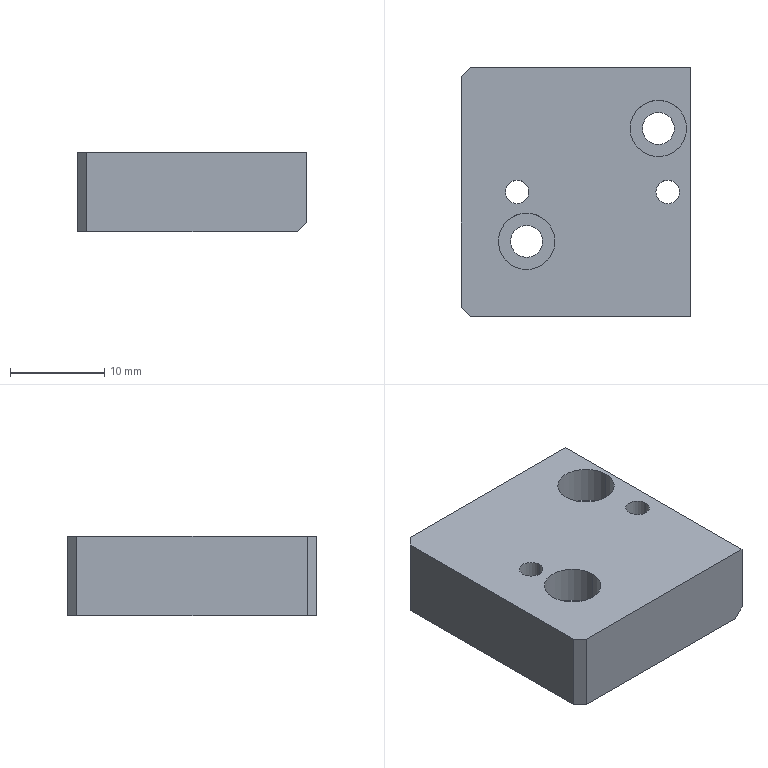Part | SolidWorks | features MoveFace 4, Chamfer 2, DelFace 2, HoleWzd 2, Extrusion 1, Fillet 1, ICE 1 | 1 solid | 30 faces | box 24.4 x 26.5 x 8.5 mm | volume 3196 mm3 | plane 16 | cylinder 14 | commonest cylinder face diameters 2.5 x4 3.4 x4 6 x4 5 x2
STEP:
#1=CARTESIAN_POINT('',(-21.3,93.75,0.));
#2=VERTEX_POINT('',#1);
#3=CARTESIAN_POINT('',(-18.8,93.75,0.));
#4=VERTEX_POINT('',#3);
#5=CARTESIAN_POINT('',(-20.05,93.75,0.));
#6=DIRECTION('',(0.,0.,1.));
#7=DIRECTION('',(1.,0.,0.));
#8=AXIS2_PLACEMENT_3D('',#5,#6,#7);
#9=CIRCLE('',#8,1.25);
#10=EDGE_CURVE('',#2,#4,#9,.T.);
#11=ORIENTED_EDGE('',*,*,#10,.F.);
#12=CARTESIAN_POINT('',(-21.3,93.75,5.));
#13=VERTEX_POINT('',#12);
#14=CARTESIAN_POINT('',(-21.3,93.75,5.));
#15=DIRECTION('',(0.,0.,1.));
#16=VECTOR('',#15,1000.);
#17=LINE('',#14,#16);
#18=EDGE_CURVE('',#2,#13,#17,.T.);
#19=ORIENTED_EDGE('',*,*,#18,.T.);
#20=CARTESIAN_POINT('',(-18.8,93.75,5.));
#21=VERTEX_POINT('',#20);
#22=CARTESIAN_POINT('',(-20.05,93.75,5.));
#23=DIRECTION('',(0.,0.,1.));
#24=DIRECTION('',(1.,0.,0.));
#25=AXIS2_PLACEMENT_3D('',#22,#23,#24);
#26=CIRCLE('',#25,1.25);
#27=EDGE_CURVE('',#13,#21,#26,.T.);
#28=ORIENTED_EDGE('',*,*,#27,.T.);
#29=CARTESIAN_POINT('',(-18.8,93.75,5.));
#30=DIRECTION('',(0.,0.,1.));
#31=VECTOR('',#30,1000.);
#32=LINE('',#29,#31);
#33=EDGE_CURVE('',#4,#21,#32,.T.);
#34=ORIENTED_EDGE('',*,*,#33,.F.);
#35=EDGE_LOOP('',(#11,#19,#28,#34));
#36=FACE_OUTER_BOUND('',#35,.T.);
#37=CARTESIAN_POINT('',(-20.05,93.75,5.));
#38=DIRECTION('',(0.,0.,1.));
#39=DIRECTION('',(1.,0.,0.));
#40=AXIS2_PLACEMENT_3D('',#37,#38,#39);
#41=CYLINDRICAL_SURFACE('',#40,1.25);
#42=ADVANCED_FACE('',(#36),#41,.F.);
#43=CARTESIAN_POINT('',(-5.3,93.75,0.));
#44=VERTEX_POINT('',#43);
#45=CARTESIAN_POINT('',(-2.8,93.75,0.));
#46=VERTEX_POINT('',#45);
#47=CARTESIAN_POINT('',(-4.05,93.75,0.));
#48=DIRECTION('',(0.,0.,1.));
#49=DIRECTION('',(1.,0.,0.));
#50=AXIS2_PLACEMENT_3D('',#47,#48,#49);
#51=CIRCLE('',#50,1.25);
#52=EDGE_CURVE('',#44,#46,#51,.T.);
#53=ORIENTED_EDGE('',*,*,#52,.F.);
#54=CARTESIAN_POINT('',(-5.3,93.75,5.));
#55=VERTEX_POINT('',#54);
#56=CARTESIAN_POINT('',(-5.3,93.75,5.));
#57=DIRECTION('',(0.,0.,1.));
#58=VECTOR('',#57,1000.);
#59=LINE('',#56,#58);
#60=EDGE_CURVE('',#44,#55,#59,.T.);
#61=ORIENTED_EDGE('',*,*,#60,.T.);
#62=CARTESIAN_POINT('',(-2.8,93.75,5.));
#63=VERTEX_POINT('',#62);
#64=CARTESIAN_POINT('',(-4.05,93.75,5.));
#65=DIRECTION('',(0.,0.,1.));
#66=DIRECTION('',(1.,0.,0.));
#67=AXIS2_PLACEMENT_3D('',#64,#65,#66);
#68=CIRCLE('',#67,1.25);
#69=EDGE_CURVE('',#55,#63,#68,.T.);
#70=ORIENTED_EDGE('',*,*,#69,.T.);
#71=CARTESIAN_POINT('',(-2.8,93.75,5.));
#72=DIRECTION('',(0.,0.,1.));
#73=VECTOR('',#72,1000.);
#74=LINE('',#71,#73);
#75=EDGE_CURVE('',#46,#63,#74,.T.);
#76=ORIENTED_EDGE('',*,*,#75,.F.);
#77=EDGE_LOOP('',(#53,#61,#70,#76));
#78=FACE_OUTER_BOUND('',#77,.T.);
#79=CARTESIAN_POINT('',(-4.05,93.75,5.));
#80=DIRECTION('',(0.,0.,1.));
#81=DIRECTION('',(1.,0.,0.));
#82=AXIS2_PLACEMENT_3D('',#79,#80,#81);
#83=CYLINDRICAL_SURFACE('',#82,1.25);
#84=ADVANCED_FACE('',(#78),#83,.F.);
#85=CARTESIAN_POINT('',(-8.05,100.5,1.));
#86=VERTEX_POINT('',#85);
#87=CARTESIAN_POINT('',(-2.05,100.5,1.));
#88=VERTEX_POINT('',#87);
#89=CARTESIAN_POINT('',(-5.05,100.5,1.));
#90=DIRECTION('',(0.,0.,1.));
#91=DIRECTION('',(1.,0.,0.));
#92=AXIS2_PLACEMENT_3D('',#89,#90,#91);
#93=CIRCLE('',#92,3.);
#94=EDGE_CURVE('',#86,#88,#93,.T.);
#95=ORIENTED_EDGE('',*,*,#94,.F.);
#96=CARTESIAN_POINT('',(-8.05,100.5,5.));
#97=VERTEX_POINT('',#96);
#98=CARTESIAN_POINT('',(-8.05,100.5,5.));
#99=DIRECTION('',(0.,0.,1.));
#100=VECTOR('',#99,1000.);
#101=LINE('',#98,#100);
#102=EDGE_CURVE('',#86,#97,#101,.T.);
#103=ORIENTED_EDGE('',*,*,#102,.T.);
#104=CARTESIAN_POINT('',(-2.05,100.5,5.));
#105=VERTEX_POINT('',#104);
#106=CARTESIAN_POINT('',(-5.05,100.5,5.));
#107=DIRECTION('',(0.,0.,1.));
#108=DIRECTION('',(1.,0.,0.));
#109=AXIS2_PLACEMENT_3D('',#106,#107,#108);
#110=CIRCLE('',#109,3.);
#111=EDGE_CURVE('',#97,#105,#110,.T.);
#112=ORIENTED_EDGE('',*,*,#111,.T.);
#113=CARTESIAN_POINT('',(-2.05,100.5,5.));
#114=DIRECTION('',(0.,0.,1.));
#115=VECTOR('',#114,1000.);
#116=LINE('',#113,#115);
#117=EDGE_CURVE('',#88,#105,#116,.T.);
#118=ORIENTED_EDGE('',*,*,#117,.F.);
#119=EDGE_LOOP('',(#95,#103,#112,#118));
#120=FACE_OUTER_BOUND('',#119,.T.);
#121=CARTESIAN_POINT('',(-5.05,100.5,5.));
#122=DIRECTION('',(0.,0.,1.));
#123=DIRECTION('',(1.,0.,0.));
#124=AXIS2_PLACEMENT_3D('',#121,#122,#123);
#125=CYLINDRICAL_SURFACE('',#124,3.);
#126=ADVANCED_FACE('',(#120),#125,.F.);
#127=CARTESIAN_POINT('',(-6.75,100.5,0.));
#128=VERTEX_POINT('',#127);
#129=CARTESIAN_POINT('',(-3.35,100.5,0.));
#130=VERTEX_POINT('',#129);
#131=CARTESIAN_POINT('',(-5.05,100.5,0.));
#132=DIRECTION('',(0.,0.,1.));
#133=DIRECTION('',(1.,0.,0.));
#134=AXIS2_PLACEMENT_3D('',#131,#132,#133);
#135=CIRCLE('',#134,1.7);
#136=EDGE_CURVE('',#128,#130,#135,.T.);
#137=ORIENTED_EDGE('',*,*,#136,.F.);
#138=CARTESIAN_POINT('',(-6.75,100.5,1.));
#139=VERTEX_POINT('',#138);
#140=CARTESIAN_POINT('',(-6.75,100.5,5.));
#141=DIRECTION('',(0.,0.,1.));
#142=VECTOR('',#141,1000.);
#143=LINE('',#140,#142);
#144=EDGE_CURVE('',#128,#139,#143,.T.);
#145=ORIENTED_EDGE('',*,*,#144,.T.);
#146=CARTESIAN_POINT('',(-3.35,100.5,1.));
#147=VERTEX_POINT('',#146);
#148=CARTESIAN_POINT('',(-5.05,100.5,1.));
#149=DIRECTION('',(0.,0.,1.));
#150=DIRECTION('',(1.,0.,0.));
#151=AXIS2_PLACEMENT_3D('',#148,#149,#150);
#152=CIRCLE('',#151,1.7);
#153=EDGE_CURVE('',#139,#147,#152,.T.);
#154=ORIENTED_EDGE('',*,*,#153,.T.);
#155=CARTESIAN_POINT('',(-3.35,100.5,5.));
#156=DIRECTION('',(0.,0.,1.));
#157=VECTOR('',#156,1000.);
#158=LINE('',#155,#157);
#159=EDGE_CURVE('',#130,#147,#158,.T.);
#160=ORIENTED_EDGE('',*,*,#159,.F.);
#161=EDGE_LOOP('',(#137,#145,#154,#160));
#162=FACE_OUTER_BOUND('',#161,.T.);
#163=CARTESIAN_POINT('',(-5.05,100.5,5.));
#164=DIRECTION('',(0.,0.,1.));
#165=DIRECTION('',(1.,0.,0.));
#166=AXIS2_PLACEMENT_3D('',#163,#164,#165);
#167=CYLINDRICAL_SURFACE('',#166,1.7);
#168=ADVANCED_FACE('',(#162),#167,.F.);
#169=CARTESIAN_POINT('',(-22.05,88.5,1.));
#170=VERTEX_POINT('',#169);
#171=CARTESIAN_POINT('',(-16.05,88.5,1.));
#172=VERTEX_POINT('',#171);
#173=CARTESIAN_POINT('',(-19.05,88.5,1.));
#174=DIRECTION('',(0.,0.,1.));
#175=DIRECTION('',(1.,0.,0.));
#176=AXIS2_PLACEMENT_3D('',#173,#174,#175);
#177=CIRCLE('',#176,3.);
#178=EDGE_CURVE('',#170,#172,#177,.T.);
#179=ORIENTED_EDGE('',*,*,#178,.F.);
#180=CARTESIAN_POINT('',(-22.05,88.5,5.));
#181=VERTEX_POINT('',#180);
#182=CARTESIAN_POINT('',(-22.05,88.5,5.));
#183=DIRECTION('',(0.,0.,1.));
#184=VECTOR('',#183,1000.);
#185=LINE('',#182,#184);
#186=EDGE_CURVE('',#170,#181,#185,.T.);
#187=ORIENTED_EDGE('',*,*,#186,.T.);
#188=CARTESIAN_POINT('',(-16.05,88.5,5.));
#189=VERTEX_POINT('',#188);
#190=CARTESIAN_POINT('',(-19.05,88.5,5.));
#191=DIRECTION('',(0.,0.,1.));
#192=DIRECTION('',(1.,0.,0.));
#193=AXIS2_PLACEMENT_3D('',#190,#191,#192);
#194=CIRCLE('',#193,3.);
#195=EDGE_CURVE('',#181,#189,#194,.T.);
#196=ORIENTED_EDGE('',*,*,#195,.T.);
#197=CARTESIAN_POINT('',(-16.05,88.5,5.));
#198=DIRECTION('',(0.,0.,1.));
#199=VECTOR('',#198,1000.);
#200=LINE('',#197,#199);
#201=EDGE_CURVE('',#172,#189,#200,.T.);
#202=ORIENTED_EDGE('',*,*,#201,.F.);
#203=EDGE_LOOP('',(#179,#187,#196,#202));
#204=FACE_OUTER_BOUND('',#203,.T.);
#205=CARTESIAN_POINT('',(-19.05,88.5,5.));
#206=DIRECTION('',(0.,0.,1.));
#207=DIRECTION('',(1.,0.,0.));
#208=AXIS2_PLACEMENT_3D('',#205,#206,#207);
#209=CYLINDRICAL_SURFACE('',#208,3.);
#210=ADVANCED_FACE('',(#204),#209,.F.);
#211=CARTESIAN_POINT('',(-20.75,88.5,0.));
#212=VERTEX_POINT('',#211);
#213=CARTESIAN_POINT('',(-17.35,88.5,0.));
#214=VERTEX_POINT('',#213);
#215=CARTESIAN_POINT('',(-19.05,88.5,0.));
#216=DIRECTION('',(0.,0.,1.));
#217=DIRECTION('',(1.,0.,0.));
#218=AXIS2_PLACEMENT_3D('',#215,#216,#217);
#219=CIRCLE('',#218,1.7);
#220=EDGE_CURVE('',#212,#214,#219,.T.);
#221=ORIENTED_EDGE('',*,*,#220,.F.);
#222=CARTESIAN_POINT('',(-20.75,88.5,1.));
#223=VERTEX_POINT('',#222);
#224=CARTESIAN_POINT('',(-20.75,88.5,5.));
#225=DIRECTION('',(0.,0.,1.));
#226=VECTOR('',#225,1000.);
#227=LINE('',#224,#226);
#228=EDGE_CURVE('',#212,#223,#227,.T.);
#229=ORIENTED_EDGE('',*,*,#228,.T.);
#230=CARTESIAN_POINT('',(-17.35,88.5,1.));
#231=VERTEX_POINT('',#230);
#232=CARTESIAN_POINT('',(-19.05,88.5,1.));
#233=DIRECTION('',(0.,0.,1.));
#234=DIRECTION('',(1.,0.,0.));
#235=AXIS2_PLACEMENT_3D('',#232,#233,#234);
#236=CIRCLE('',#235,1.7);
#237=EDGE_CURVE('',#223,#231,#236,.T.);
#238=ORIENTED_EDGE('',*,*,#237,.T.);
#239=CARTESIAN_POINT('',(-17.35,88.5,5.));
#240=DIRECTION('',(0.,0.,1.));
#241=VECTOR('',#240,1000.);
#242=LINE('',#239,#241);
#243=EDGE_CURVE('',#214,#231,#242,.T.);
#244=ORIENTED_EDGE('',*,*,#243,.F.);
#245=EDGE_LOOP('',(#221,#229,#238,#244));
#246=FACE_OUTER_BOUND('',#245,.T.);
#247=CARTESIAN_POINT('',(-19.05,88.5,5.));
#248=DIRECTION('',(0.,0.,1.));
#249=DIRECTION('',(1.,0.,0.));
#250=AXIS2_PLACEMENT_3D('',#247,#248,#249);
#251=CYLINDRICAL_SURFACE('',#250,1.7);
#252=ADVANCED_FACE('',(#246),#251,.F.);
#253=CARTESIAN_POINT('',(-19.05,88.5,0.));
#254=DIRECTION('',(0.,0.,1.));
#255=DIRECTION('',(1.,0.,0.));
#256=AXIS2_PLACEMENT_3D('',#253,#254,#255);
#257=CIRCLE('',#256,1.7);
#258=EDGE_CURVE('',#214,#212,#257,.T.);
#259=ORIENTED_EDGE('',*,*,#258,.T.);
#260=ORIENTED_EDGE('',*,*,#220,.T.);
#261=EDGE_LOOP('',(#259,#260));
#262=FACE_BOUND('',#261,.T.);
#263=CARTESIAN_POINT('',(-5.05,100.5,0.));
#264=DIRECTION('',(0.,0.,1.));
#265=DIRECTION('',(1.,0.,0.));
#266=AXIS2_PLACEMENT_3D('',#263,#264,#265);
#267=CIRCLE('',#266,1.7);
#268=EDGE_CURVE('',#130,#128,#267,.T.);
#269=ORIENTED_EDGE('',*,*,#268,.T.);
#270=ORIENTED_EDGE('',*,*,#136,.T.);
#271=EDGE_LOOP('',(#269,#270));
#272=FACE_BOUND('',#271,.T.);
#273=CARTESIAN_POINT('',(-4.05,93.75,0.));
#274=DIRECTION('',(0.,0.,1.));
#275=DIRECTION('',(1.,0.,0.));
#276=AXIS2_PLACEMENT_3D('',#273,#274,#275);
#277=CIRCLE('',#276,1.25);
#278=EDGE_CURVE('',#46,#44,#277,.T.);
#279=ORIENTED_EDGE('',*,*,#278,.T.);
#280=ORIENTED_EDGE('',*,*,#52,.T.);
#281=EDGE_LOOP('',(#279,#280));
#282=FACE_BOUND('',#281,.T.);
#283=CARTESIAN_POINT('',(-20.05,93.75,0.));
#284=DIRECTION('',(0.,0.,1.));
#285=DIRECTION('',(1.,0.,0.));
#286=AXIS2_PLACEMENT_3D('',#283,#284,#285);
#287=CIRCLE('',#286,1.25);
#288=EDGE_CURVE('',#4,#2,#287,.T.);
#289=ORIENTED_EDGE('',*,*,#288,.T.);
#290=ORIENTED_EDGE('',*,*,#10,.T.);
#291=EDGE_LOOP('',(#289,#290));
#292=FACE_BOUND('',#291,.T.);
#293=CARTESIAN_POINT('',(-22.5,81.5,0.));
#294=VERTEX_POINT('',#293);
#295=CARTESIAN_POINT('',(-1.6,81.5,0.));
#296=VERTEX_POINT('',#295);
#297=CARTESIAN_POINT('',(-25.,81.5,0.));
#298=DIRECTION('',(1.,0.,0.));
#299=VECTOR('',#298,1000.);
#300=LINE('',#297,#299);
#301=EDGE_CURVE('',#294,#296,#300,.T.);
#302=ORIENTED_EDGE('',*,*,#301,.F.);
#303=CARTESIAN_POINT('',(-25.,84.,0.));
#304=VERTEX_POINT('',#303);
#305=CARTESIAN_POINT('',(-22.5,84.,0.));
#306=DIRECTION('',(0.,0.,-1.));
#307=DIRECTION('',(1.,0.,0.));
#308=AXIS2_PLACEMENT_3D('',#305,#306,#307);
#309=CIRCLE('',#308,2.5);
#310=EDGE_CURVE('',#294,#304,#309,.T.);
#311=ORIENTED_EDGE('',*,*,#310,.T.);
#312=CARTESIAN_POINT('',(-25.,103.5,0.));
#313=VERTEX_POINT('',#312);
#314=CARTESIAN_POINT('',(-25.,106.,0.));
#315=DIRECTION('',(0.,-1.,0.));
#316=VECTOR('',#315,1000.);
#317=LINE('',#314,#316);
#318=EDGE_CURVE('',#313,#304,#317,.T.);
#319=ORIENTED_EDGE('',*,*,#318,.F.);
#320=CARTESIAN_POINT('',(-22.5,106.,0.));
#321=VERTEX_POINT('',#320);
#322=CARTESIAN_POINT('',(-22.5,103.5,0.));
#323=DIRECTION('',(0.,0.,-1.));
#324=DIRECTION('',(1.,0.,0.));
#325=AXIS2_PLACEMENT_3D('',#322,#323,#324);
#326=CIRCLE('',#325,2.5);
#327=EDGE_CURVE('',#313,#321,#326,.T.);
#328=ORIENTED_EDGE('',*,*,#327,.T.);
#329=CARTESIAN_POINT('',(-1.6,106.,0.));
#330=VERTEX_POINT('',#329);
#331=CARTESIAN_POINT('',(-1.6,106.,0.));
#332=DIRECTION('',(-1.,0.,0.));
#333=VECTOR('',#332,1000.);
#334=LINE('',#331,#333);
#335=EDGE_CURVE('',#330,#321,#334,.T.);
#336=ORIENTED_EDGE('',*,*,#335,.F.);
#337=CARTESIAN_POINT('',(-1.6,97.5,0.));
#338=DIRECTION('',(0.,1.,0.));
#339=VECTOR('',#338,1000.);
#340=LINE('',#337,#339);
#341=EDGE_CURVE('',#296,#330,#340,.T.);
#342=ORIENTED_EDGE('',*,*,#341,.F.);
#343=EDGE_LOOP('',(#302,#311,#319,#328,#336,#342));
#344=FACE_OUTER_BOUND('',#343,.T.);
#345=CARTESIAN_POINT('',(0.,0.,0.));
#346=DIRECTION('',(0.,0.,1.));
#347=DIRECTION('',(1.,0.,0.));
#348=AXIS2_PLACEMENT_3D('',#345,#346,#347);
#349=PLANE('',#348);
#350=ADVANCED_FACE('',(#262,#272,#282,#292,#344),#349,.F.);
#351=CARTESIAN_POINT('',(-25.,107.,5.));
#352=VERTEX_POINT('',#351);
#353=CARTESIAN_POINT('',(-25.,107.,-3.5));
#354=VERTEX_POINT('',#353);
#355=CARTESIAN_POINT('',(-25.,107.,5.));
#356=DIRECTION('',(0.,0.,-1.));
#357=VECTOR('',#356,1000.);
#358=LINE('',#355,#357);
#359=EDGE_CURVE('',#352,#354,#358,.T.);
#360=ORIENTED_EDGE('',*,*,#359,.T.);
#361=CARTESIAN_POINT('',(-26.,106.,-3.5));
#362=VERTEX_POINT('',#361);
#363=CARTESIAN_POINT('',(-25.,107.,-3.5));
#364=DIRECTION('',(0.7071,0.7071,0.));
#365=VECTOR('',#364,1000.);
#366=LINE('',#363,#365);
#367=EDGE_CURVE('',#362,#354,#366,.T.);
#368=ORIENTED_EDGE('',*,*,#367,.F.);
#369=CARTESIAN_POINT('',(-26.,106.,5.));
#370=VERTEX_POINT('',#369);
#371=CARTESIAN_POINT('',(-26.,106.,5.));
#372=DIRECTION('',(0.,0.,-1.));
#373=VECTOR('',#372,1000.);
#374=LINE('',#371,#373);
#375=EDGE_CURVE('',#370,#362,#374,.T.);
#376=ORIENTED_EDGE('',*,*,#375,.F.);
#377=CARTESIAN_POINT('',(-25.,107.,5.));
#378=DIRECTION('',(-0.7071,-0.7071,0.));
#379=VECTOR('',#378,1000.);
#380=LINE('',#377,#379);
#381=EDGE_CURVE('',#352,#370,#380,.T.);
#382=ORIENTED_EDGE('',*,*,#381,.F.);
#383=EDGE_LOOP('',(#360,#368,#376,#382));
#384=FACE_OUTER_BOUND('',#383,.T.);
#385=CARTESIAN_POINT('',(-25.,107.,5.));
#386=DIRECTION('',(0.7071,-0.7071,0.));
#387=DIRECTION('',(0.7071,0.7071,0.));
#388=AXIS2_PLACEMENT_3D('',#385,#386,#387);
#389=PLANE('',#388);
#390=ADVANCED_FACE('',(#384),#389,.F.);
#391=ORIENTED_EDGE('',*,*,#375,.T.);
#392=CARTESIAN_POINT('',(-26.,81.5,-3.5));
#393=VERTEX_POINT('',#392);
#394=CARTESIAN_POINT('',(-26.,106.,-3.5));
#395=DIRECTION('',(0.,1.,0.));
#396=VECTOR('',#395,1000.);
#397=LINE('',#394,#396);
#398=EDGE_CURVE('',#393,#362,#397,.T.);
#399=ORIENTED_EDGE('',*,*,#398,.F.);
#400=CARTESIAN_POINT('',(-26.,81.5,5.));
#401=VERTEX_POINT('',#400);
#402=CARTESIAN_POINT('',(-26.,81.5,5.));
#403=DIRECTION('',(0.,0.,-1.));
#404=VECTOR('',#403,1000.);
#405=LINE('',#402,#404);
#406=EDGE_CURVE('',#401,#393,#405,.T.);
#407=ORIENTED_EDGE('',*,*,#406,.F.);
#408=CARTESIAN_POINT('',(-26.,103.5,5.));
#409=DIRECTION('',(0.,-1.,0.));
#410=VECTOR('',#409,1000.);
#411=LINE('',#408,#410);
#412=EDGE_CURVE('',#370,#401,#411,.T.);
#413=ORIENTED_EDGE('',*,*,#412,.F.);
#414=EDGE_LOOP('',(#391,#399,#407,#413));
#415=FACE_OUTER_BOUND('',#414,.T.);
#416=CARTESIAN_POINT('',(-26.,103.5,5.));
#417=DIRECTION('',(1.,0.,0.));
#418=DIRECTION('',(0.,1.,0.));
#419=AXIS2_PLACEMENT_3D('',#416,#417,#418);
#420=PLANE('',#419);
#421=ADVANCED_FACE('',(#415),#420,.F.);
#422=ORIENTED_EDGE('',*,*,#406,.T.);
#423=CARTESIAN_POINT('',(-25.,80.5,-3.5));
#424=VERTEX_POINT('',#423);
#425=CARTESIAN_POINT('',(-26.,81.5,-3.5));
#426=DIRECTION('',(-0.7071,0.7071,0.));
#427=VECTOR('',#426,1000.);
#428=LINE('',#425,#427);
#429=EDGE_CURVE('',#424,#393,#428,.T.);
#430=ORIENTED_EDGE('',*,*,#429,.F.);
#431=CARTESIAN_POINT('',(-25.,80.5,5.));
#432=VERTEX_POINT('',#431);
#433=CARTESIAN_POINT('',(-25.,80.5,5.));
#434=DIRECTION('',(0.,0.,-1.));
#435=VECTOR('',#434,1000.);
#436=LINE('',#433,#435);
#437=EDGE_CURVE('',#432,#424,#436,.T.);
#438=ORIENTED_EDGE('',*,*,#437,.F.);
#439=CARTESIAN_POINT('',(-26.,81.5,5.));
#440=DIRECTION('',(0.7071,-0.7071,0.));
#441=VECTOR('',#440,1000.);
#442=LINE('',#439,#441);
#443=EDGE_CURVE('',#401,#432,#442,.T.);
#444=ORIENTED_EDGE('',*,*,#443,.F.);
#445=EDGE_LOOP('',(#422,#430,#438,#444));
#446=FACE_OUTER_BOUND('',#445,.T.);
#447=CARTESIAN_POINT('',(-26.,81.5,5.));
#448=DIRECTION('',(0.7071,0.7071,0.));
#449=DIRECTION('',(-0.7071,0.7071,0.));
#450=AXIS2_PLACEMENT_3D('',#447,#448,#449);
#451=PLANE('',#450);
#452=ADVANCED_FACE('',(#446),#451,.F.);
#453=CARTESIAN_POINT('',(-2.6,80.5,-3.5));
#454=VERTEX_POINT('',#453);
#455=CARTESIAN_POINT('',(-25.,80.5,-3.5));
#456=DIRECTION('',(-1.,0.,0.));
#457=VECTOR('',#456,1000.);
#458=LINE('',#455,#457);
#459=EDGE_CURVE('',#454,#424,#458,.T.);
#460=ORIENTED_EDGE('',*,*,#459,.F.);
#461=CARTESIAN_POINT('',(-1.6,80.5,-2.5));
#462=VERTEX_POINT('',#461);
#463=CARTESIAN_POINT('',(-2.6,80.5,-3.5));
#464=DIRECTION('',(0.7071,0.,0.7071));
#465=VECTOR('',#464,1000.);
#466=LINE('',#463,#465);
#467=EDGE_CURVE('',#454,#462,#466,.T.);
#468=ORIENTED_EDGE('',*,*,#467,.T.);
#469=CARTESIAN_POINT('',(-1.6,80.5,5.));
#470=VERTEX_POINT('',#469);
#471=CARTESIAN_POINT('',(-1.6,80.5,5.));
#472=DIRECTION('',(0.,0.,1.));
#473=VECTOR('',#472,1000.);
#474=LINE('',#471,#473);
#475=EDGE_CURVE('',#462,#470,#474,.T.);
#476=ORIENTED_EDGE('',*,*,#475,.T.);
#477=CARTESIAN_POINT('',(-22.5,80.5,5.));
#478=DIRECTION('',(1.,0.,0.));
#479=VECTOR('',#478,1000.);
#480=LINE('',#477,#479);
#481=EDGE_CURVE('',#432,#470,#480,.T.);
#482=ORIENTED_EDGE('',*,*,#481,.F.);
#483=ORIENTED_EDGE('',*,*,#437,.T.);
#484=EDGE_LOOP('',(#460,#468,#476,#482,#483));
#485=FACE_OUTER_BOUND('',#484,.T.);
#486=CARTESIAN_POINT('',(-22.5,80.5,5.));
#487=DIRECTION('',(0.,1.,0.));
#488=DIRECTION('',(0.,0.,1.));
#489=AXIS2_PLACEMENT_3D('',#486,#487,#488);
#490=PLANE('',#489);
#491=ADVANCED_FACE('',(#485),#490,.F.);
#492=ORIENTED_EDGE('',*,*,#475,.F.);
#493=CARTESIAN_POINT('',(-1.6,81.5,-2.5));
#494=VERTEX_POINT('',#493);
#495=CARTESIAN_POINT('',(-1.6,81.5,-2.5));
#496=DIRECTION('',(0.,1.,0.));
#497=VECTOR('',#496,1000.);
#498=LINE('',#495,#497);
#499=EDGE_CURVE('',#462,#494,#498,.T.);
#500=ORIENTED_EDGE('',*,*,#499,.T.);
#501=CARTESIAN_POINT('',(-1.6,81.5,-3.5));
#502=DIRECTION('',(0.,0.,1.));
#503=VECTOR('',#502,1000.);
#504=LINE('',#501,#503);
#505=EDGE_CURVE('',#494,#296,#504,.T.);
#506=ORIENTED_EDGE('',*,*,#505,.T.);
#507=ORIENTED_EDGE('',*,*,#341,.T.);
#508=CARTESIAN_POINT('',(-1.6,106.,-2.5));
#509=VERTEX_POINT('',#508);
#510=CARTESIAN_POINT('',(-1.6,106.,-3.5));
#511=DIRECTION('',(0.,0.,1.));
#512=VECTOR('',#511,1000.);
#513=LINE('',#510,#512);
#514=EDGE_CURVE('',#509,#330,#513,.T.);
#515=ORIENTED_EDGE('',*,*,#514,.F.);
#516=CARTESIAN_POINT('',(-1.6,107.,-2.5));
#517=VERTEX_POINT('',#516);
#518=CARTESIAN_POINT('',(-1.6,107.,-2.5));
#519=DIRECTION('',(0.,1.,0.));
#520=VECTOR('',#519,1000.);
#521=LINE('',#518,#520);
#522=EDGE_CURVE('',#509,#517,#521,.T.);
#523=ORIENTED_EDGE('',*,*,#522,.T.);
#524=CARTESIAN_POINT('',(-1.6,107.,5.));
#525=VERTEX_POINT('',#524);
#526=CARTESIAN_POINT('',(-1.6,107.,5.));
#527=DIRECTION('',(0.,0.,-1.));
#528=VECTOR('',#527,1000.);
#529=LINE('',#526,#528);
#530=EDGE_CURVE('',#525,#517,#529,.T.);
#531=ORIENTED_EDGE('',*,*,#530,.F.);
#532=CARTESIAN_POINT('',(-1.6,97.5,5.));
#533=DIRECTION('',(0.,1.,0.));
#534=VECTOR('',#533,1000.);
#535=LINE('',#532,#534);
#536=EDGE_CURVE('',#470,#525,#535,.T.);
#537=ORIENTED_EDGE('',*,*,#536,.F.);
#538=EDGE_LOOP('',(#492,#500,#506,#507,#515,#523,#531,#537));
#539=FACE_OUTER_BOUND('',#538,.T.);
#540=CARTESIAN_POINT('',(-1.6,97.5,5.));
#541=DIRECTION('',(-1.,0.,0.));
#542=DIRECTION('',(0.,-1.,0.));
#543=AXIS2_PLACEMENT_3D('',#540,#541,#542);
#544=PLANE('',#543);
#545=ADVANCED_FACE('',(#539),#544,.F.);
#546=ORIENTED_EDGE('',*,*,#530,.T.);
#547=CARTESIAN_POINT('',(-2.6,107.,-3.5));
#548=VERTEX_POINT('',#547);
#549=CARTESIAN_POINT('',(-2.6,107.,-3.5));
#550=DIRECTION('',(-0.7071,0.,-0.7071));
#551=VECTOR('',#550,1000.);
#552=LINE('',#549,#551);
#553=EDGE_CURVE('',#517,#548,#552,.T.);
#554=ORIENTED_EDGE('',*,*,#553,.T.);
#555=CARTESIAN_POINT('',(-1.6,107.,-3.5));
#556=DIRECTION('',(1.,0.,0.));
#557=VECTOR('',#556,1000.);
#558=LINE('',#555,#557);
#559=EDGE_CURVE('',#354,#548,#558,.T.);
#560=ORIENTED_EDGE('',*,*,#559,.F.);
#561=ORIENTED_EDGE('',*,*,#359,.F.);
#562=CARTESIAN_POINT('',(-2.6,107.,5.));
#563=DIRECTION('',(-1.,0.,0.));
#564=VECTOR('',#563,1000.);
#565=LINE('',#562,#564);
#566=EDGE_CURVE('',#525,#352,#565,.T.);
#567=ORIENTED_EDGE('',*,*,#566,.F.);
#568=EDGE_LOOP('',(#546,#554,#560,#561,#567));
#569=FACE_OUTER_BOUND('',#568,.T.);
#570=CARTESIAN_POINT('',(-2.6,107.,5.));
#571=DIRECTION('',(0.,-1.,0.));
#572=DIRECTION('',(0.,0.,-1.));
#573=AXIS2_PLACEMENT_3D('',#570,#571,#572);
#574=PLANE('',#573);
#575=ADVANCED_FACE('',(#569),#574,.F.);
#576=CARTESIAN_POINT('',(-20.05,93.75,5.));
#577=DIRECTION('',(0.,0.,1.));
#578=DIRECTION('',(1.,0.,0.));
#579=AXIS2_PLACEMENT_3D('',#576,#577,#578);
#580=CIRCLE('',#579,1.25);
#581=EDGE_CURVE('',#21,#13,#580,.T.);
#582=ORIENTED_EDGE('',*,*,#581,.F.);
#583=ORIENTED_EDGE('',*,*,#27,.F.);
#584=EDGE_LOOP('',(#582,#583));
#585=FACE_BOUND('',#584,.T.);
#586=CARTESIAN_POINT('',(-4.05,93.75,5.));
#587=DIRECTION('',(0.,0.,1.));
#588=DIRECTION('',(1.,0.,0.));
#589=AXIS2_PLACEMENT_3D('',#586,#587,#588);
#590=CIRCLE('',#589,1.25);
#591=EDGE_CURVE('',#63,#55,#590,.T.);
#592=ORIENTED_EDGE('',*,*,#591,.F.);
#593=ORIENTED_EDGE('',*,*,#69,.F.);
#594=EDGE_LOOP('',(#592,#593));
#595=FACE_BOUND('',#594,.T.);
#596=ORIENTED_EDGE('',*,*,#481,.T.);
#597=ORIENTED_EDGE('',*,*,#536,.T.);
#598=ORIENTED_EDGE('',*,*,#566,.T.);
#599=ORIENTED_EDGE('',*,*,#381,.T.);
#600=ORIENTED_EDGE('',*,*,#412,.T.);
#601=ORIENTED_EDGE('',*,*,#443,.T.);
#602=EDGE_LOOP('',(#596,#597,#598,#599,#600,#601));
#603=FACE_OUTER_BOUND('',#602,.T.);
#604=CARTESIAN_POINT('',(-5.05,100.5,5.));
#605=DIRECTION('',(0.,0.,1.));
#606=DIRECTION('',(1.,0.,0.));
#607=AXIS2_PLACEMENT_3D('',#604,#605,#606);
#608=CIRCLE('',#607,3.);
#609=EDGE_CURVE('',#105,#97,#608,.T.);
#610=ORIENTED_EDGE('',*,*,#609,.F.);
#611=ORIENTED_EDGE('',*,*,#111,.F.);
#612=EDGE_LOOP('',(#610,#611));
#613=FACE_BOUND('',#612,.T.);
#614=CARTESIAN_POINT('',(-19.05,88.5,5.));
#615=DIRECTION('',(0.,0.,1.));
#616=DIRECTION('',(1.,0.,0.));
#617=AXIS2_PLACEMENT_3D('',#614,#615,#616);
#618=CIRCLE('',#617,3.);
#619=EDGE_CURVE('',#189,#181,#618,.T.);
#620=ORIENTED_EDGE('',*,*,#619,.F.);
#621=ORIENTED_EDGE('',*,*,#195,.F.);
#622=EDGE_LOOP('',(#620,#621));
#623=FACE_BOUND('',#622,.T.);
#624=CARTESIAN_POINT('',(0.,0.,5.));
#625=DIRECTION('',(0.,0.,1.));
#626=DIRECTION('',(1.,0.,0.));
#627=AXIS2_PLACEMENT_3D('',#624,#625,#626);
#628=PLANE('',#627);
#629=ADVANCED_FACE('',(#585,#595,#603,#613,#623),#628,.T.);
#630=ORIENTED_EDGE('',*,*,#228,.F.);
#631=ORIENTED_EDGE('',*,*,#258,.F.);
#632=ORIENTED_EDGE('',*,*,#243,.T.);
#633=CARTESIAN_POINT('',(-19.05,88.5,1.));
#634=DIRECTION('',(0.,0.,1.));
#635=DIRECTION('',(1.,0.,0.));
#636=AXIS2_PLACEMENT_3D('',#633,#634,#635);
#637=CIRCLE('',#636,1.7);
#638=EDGE_CURVE('',#231,#223,#637,.T.);
#639=ORIENTED_EDGE('',*,*,#638,.T.);
#640=EDGE_LOOP('',(#630,#631,#632,#639));
#641=FACE_OUTER_BOUND('',#640,.T.);
#642=CARTESIAN_POINT('',(-19.05,88.5,5.));
#643=DIRECTION('',(0.,0.,1.));
#644=DIRECTION('',(1.,0.,0.));
#645=AXIS2_PLACEMENT_3D('',#642,#643,#644);
#646=CYLINDRICAL_SURFACE('',#645,1.7);
#647=ADVANCED_FACE('',(#641),#646,.F.);
#648=ORIENTED_EDGE('',*,*,#638,.F.);
#649=ORIENTED_EDGE('',*,*,#237,.F.);
#650=EDGE_LOOP('',(#648,#649));
#651=FACE_BOUND('',#650,.T.);
#652=CARTESIAN_POINT('',(-19.05,88.5,1.));
#653=DIRECTION('',(0.,0.,1.));
#654=DIRECTION('',(1.,0.,0.));
#655=AXIS2_PLACEMENT_3D('',#652,#653,#654);
#656=CIRCLE('',#655,3.);
#657=EDGE_CURVE('',#172,#170,#656,.T.);
#658=ORIENTED_EDGE('',*,*,#657,.T.);
#659=ORIENTED_EDGE('',*,*,#178,.T.);
#660=EDGE_LOOP('',(#658,#659));
#661=FACE_OUTER_BOUND('',#660,.T.);
#662=CARTESIAN_POINT('',(-17.35,88.5,1.));
#663=DIRECTION('',(0.,0.,-1.));
#664=DIRECTION('',(-1.,0.,0.));
#665=AXIS2_PLACEMENT_3D('',#662,#663,#664);
#666=PLANE('',#665);
#667=ADVANCED_FACE('',(#651,#661),#666,.F.);
#668=ORIENTED_EDGE('',*,*,#186,.F.);
#669=ORIENTED_EDGE('',*,*,#657,.F.);
#670=ORIENTED_EDGE('',*,*,#201,.T.);
#671=ORIENTED_EDGE('',*,*,#619,.T.);
#672=EDGE_LOOP('',(#668,#669,#670,#671));
#673=FACE_OUTER_BOUND('',#672,.T.);
#674=CARTESIAN_POINT('',(-19.05,88.5,5.));
#675=DIRECTION('',(0.,0.,1.));
#676=DIRECTION('',(1.,0.,0.));
#677=AXIS2_PLACEMENT_3D('',#674,#675,#676);
#678=CYLINDRICAL_SURFACE('',#677,3.);
#679=ADVANCED_FACE('',(#673),#678,.F.);
#680=ORIENTED_EDGE('',*,*,#144,.F.);
#681=ORIENTED_EDGE('',*,*,#268,.F.);
#682=ORIENTED_EDGE('',*,*,#159,.T.);
#683=CARTESIAN_POINT('',(-5.05,100.5,1.));
#684=DIRECTION('',(0.,0.,1.));
#685=DIRECTION('',(1.,0.,0.));
#686=AXIS2_PLACEMENT_3D('',#683,#684,#685);
#687=CIRCLE('',#686,1.7);
#688=EDGE_CURVE('',#147,#139,#687,.T.);
#689=ORIENTED_EDGE('',*,*,#688,.T.);
#690=EDGE_LOOP('',(#680,#681,#682,#689));
#691=FACE_OUTER_BOUND('',#690,.T.);
#692=CARTESIAN_POINT('',(-5.05,100.5,5.));
#693=DIRECTION('',(0.,0.,1.));
#694=DIRECTION('',(1.,0.,0.));
#695=AXIS2_PLACEMENT_3D('',#692,#693,#694);
#696=CYLINDRICAL_SURFACE('',#695,1.7);
#697=ADVANCED_FACE('',(#691),#696,.F.);
#698=ORIENTED_EDGE('',*,*,#688,.F.);
#699=ORIENTED_EDGE('',*,*,#153,.F.);
#700=EDGE_LOOP('',(#698,#699));
#701=FACE_BOUND('',#700,.T.);
#702=CARTESIAN_POINT('',(-5.05,100.5,1.));
#703=DIRECTION('',(0.,0.,1.));
#704=DIRECTION('',(1.,0.,0.));
#705=AXIS2_PLACEMENT_3D('',#702,#703,#704);
#706=CIRCLE('',#705,3.);
#707=EDGE_CURVE('',#88,#86,#706,.T.);
#708=ORIENTED_EDGE('',*,*,#707,.T.);
#709=ORIENTED_EDGE('',*,*,#94,.T.);
#710=EDGE_LOOP('',(#708,#709));
#711=FACE_OUTER_BOUND('',#710,.T.);
#712=CARTESIAN_POINT('',(-3.35,100.5,1.));
#713=DIRECTION('',(0.,0.,-1.));
#714=DIRECTION('',(-1.,0.,0.));
#715=AXIS2_PLACEMENT_3D('',#712,#713,#714);
#716=PLANE('',#715);
#717=ADVANCED_FACE('',(#701,#711),#716,.F.);
#718=ORIENTED_EDGE('',*,*,#102,.F.);
#719=ORIENTED_EDGE('',*,*,#707,.F.);
#720=ORIENTED_EDGE('',*,*,#117,.T.);
#721=ORIENTED_EDGE('',*,*,#609,.T.);
#722=EDGE_LOOP('',(#718,#719,#720,#721));
#723=FACE_OUTER_BOUND('',#722,.T.);
#724=CARTESIAN_POINT('',(-5.05,100.5,5.));
#725=DIRECTION('',(0.,0.,1.));
#726=DIRECTION('',(1.,0.,0.));
#727=AXIS2_PLACEMENT_3D('',#724,#725,#726);
#728=CYLINDRICAL_SURFACE('',#727,3.);
#729=ADVANCED_FACE('',(#723),#728,.F.);
#730=ORIENTED_EDGE('',*,*,#60,.F.);
#731=ORIENTED_EDGE('',*,*,#278,.F.);
#732=ORIENTED_EDGE('',*,*,#75,.T.);
#733=ORIENTED_EDGE('',*,*,#591,.T.);
#734=EDGE_LOOP('',(#730,#731,#732,#733));
#735=FACE_OUTER_BOUND('',#734,.T.);
#736=CARTESIAN_POINT('',(-4.05,93.75,5.));
#737=DIRECTION('',(0.,0.,1.));
#738=DIRECTION('',(1.,0.,0.));
#739=AXIS2_PLACEMENT_3D('',#736,#737,#738);
#740=CYLINDRICAL_SURFACE('',#739,1.25);
#741=ADVANCED_FACE('',(#735),#740,.F.);
#742=ORIENTED_EDGE('',*,*,#18,.F.);
#743=ORIENTED_EDGE('',*,*,#288,.F.);
#744=ORIENTED_EDGE('',*,*,#33,.T.);
#745=ORIENTED_EDGE('',*,*,#581,.T.);
#746=EDGE_LOOP('',(#742,#743,#744,#745));
#747=FACE_OUTER_BOUND('',#746,.T.);
#748=CARTESIAN_POINT('',(-20.05,93.75,5.));
#749=DIRECTION('',(0.,0.,1.));
#750=DIRECTION('',(1.,0.,0.));
#751=AXIS2_PLACEMENT_3D('',#748,#749,#750);
#752=CYLINDRICAL_SURFACE('',#751,1.25);
#753=ADVANCED_FACE('',(#747),#752,.F.);
#754=CARTESIAN_POINT('',(-2.6,106.,-3.5));
#755=VERTEX_POINT('',#754);
#756=CARTESIAN_POINT('',(-22.5,106.,-3.5));
#757=VERTEX_POINT('',#756);
#758=CARTESIAN_POINT('',(-1.6,106.,-3.5));
#759=DIRECTION('',(-1.,0.,0.));
#760=VECTOR('',#759,1000.);
#761=LINE('',#758,#760);
#762=EDGE_CURVE('',#755,#757,#761,.T.);
#763=ORIENTED_EDGE('',*,*,#762,.F.);
#764=CARTESIAN_POINT('',(-2.6,106.,-3.5));
#765=DIRECTION('',(0.7071,0.,0.7071));
#766=VECTOR('',#765,1000.);
#767=LINE('',#764,#766);
#768=EDGE_CURVE('',#755,#509,#767,.T.);
#769=ORIENTED_EDGE('',*,*,#768,.T.);
#770=ORIENTED_EDGE('',*,*,#514,.T.);
#771=ORIENTED_EDGE('',*,*,#335,.T.);
#772=CARTESIAN_POINT('',(-22.5,106.,-3.5));
#773=DIRECTION('',(0.,0.,-1.));
#774=VECTOR('',#773,1000.);
#775=LINE('',#772,#774);
#776=EDGE_CURVE('',#321,#757,#775,.T.);
#777=ORIENTED_EDGE('',*,*,#776,.T.);
#778=EDGE_LOOP('',(#763,#769,#770,#771,#777));
#779=FACE_OUTER_BOUND('',#778,.T.);
#780=CARTESIAN_POINT('',(-1.6,106.,-3.5));
#781=DIRECTION('',(0.,1.,0.));
#782=DIRECTION('',(0.,0.,1.));
#783=AXIS2_PLACEMENT_3D('',#780,#781,#782);
#784=PLANE('',#783);
#785=ADVANCED_FACE('',(#779),#784,.F.);
#786=ORIENTED_EDGE('',*,*,#318,.T.);
#787=CARTESIAN_POINT('',(-25.,84.,-3.5));
#788=VERTEX_POINT('',#787);
#789=CARTESIAN_POINT('',(-25.,84.,-3.5));
#790=DIRECTION('',(0.,0.,-1.));
#791=VECTOR('',#790,1000.);
#792=LINE('',#789,#791);
#793=EDGE_CURVE('',#304,#788,#792,.T.);
#794=ORIENTED_EDGE('',*,*,#793,.T.);
#795=CARTESIAN_POINT('',(-25.,103.5,-3.5));
#796=VERTEX_POINT('',#795);
#797=CARTESIAN_POINT('',(-25.,106.,-3.5));
#798=DIRECTION('',(0.,-1.,0.));
#799=VECTOR('',#798,1000.);
#800=LINE('',#797,#799);
#801=EDGE_CURVE('',#796,#788,#800,.T.);
#802=ORIENTED_EDGE('',*,*,#801,.F.);
#803=CARTESIAN_POINT('',(-25.,103.5,0.));
#804=DIRECTION('',(0.,0.,1.));
#805=VECTOR('',#804,1000.);
#806=LINE('',#803,#805);
#807=EDGE_CURVE('',#796,#313,#806,.T.);
#808=ORIENTED_EDGE('',*,*,#807,.T.);
#809=EDGE_LOOP('',(#786,#794,#802,#808));
#810=FACE_OUTER_BOUND('',#809,.T.);
#811=CARTESIAN_POINT('',(-25.,106.,-3.5));
#812=DIRECTION('',(-1.,0.,0.));
#813=DIRECTION('',(0.,0.,1.));
#814=AXIS2_PLACEMENT_3D('',#811,#812,#813);
#815=PLANE('',#814);
#816=ADVANCED_FACE('',(#810),#815,.F.);
#817=ORIENTED_EDGE('',*,*,#505,.F.);
#818=CARTESIAN_POINT('',(-2.6,81.5,-3.5));
#819=VERTEX_POINT('',#818);
#820=CARTESIAN_POINT('',(-2.6,81.5,-3.5));
#821=DIRECTION('',(-0.7071,0.,-0.7071));
#822=VECTOR('',#821,1000.);
#823=LINE('',#820,#822);
#824=EDGE_CURVE('',#494,#819,#823,.T.);
#825=ORIENTED_EDGE('',*,*,#824,.T.);
#826=CARTESIAN_POINT('',(-22.5,81.5,-3.5));
#827=VERTEX_POINT('',#826);
#828=CARTESIAN_POINT('',(-25.,81.5,-3.5));
#829=DIRECTION('',(1.,0.,0.));
#830=VECTOR('',#829,1000.);
#831=LINE('',#828,#830);
#832=EDGE_CURVE('',#827,#819,#831,.T.);
#833=ORIENTED_EDGE('',*,*,#832,.F.);
#834=CARTESIAN_POINT('',(-22.5,81.5,0.));
#835=DIRECTION('',(0.,0.,1.));
#836=VECTOR('',#835,1000.);
#837=LINE('',#834,#836);
#838=EDGE_CURVE('',#827,#294,#837,.T.);
#839=ORIENTED_EDGE('',*,*,#838,.T.);
#840=ORIENTED_EDGE('',*,*,#301,.T.);
#841=EDGE_LOOP('',(#817,#825,#833,#839,#840));
#842=FACE_OUTER_BOUND('',#841,.T.);
#843=CARTESIAN_POINT('',(-25.,81.5,-3.5));
#844=DIRECTION('',(0.,-1.,0.));
#845=DIRECTION('',(0.,0.,-1.));
#846=AXIS2_PLACEMENT_3D('',#843,#844,#845);
#847=PLANE('',#846);
#848=ADVANCED_FACE('',(#842),#847,.F.);
#849=ORIENTED_EDGE('',*,*,#832,.T.);
#850=CARTESIAN_POINT('',(-2.6,80.5,-3.5));
#851=DIRECTION('',(0.,-1.,0.));
#852=VECTOR('',#851,1000.);
#853=LINE('',#850,#852);
#854=EDGE_CURVE('',#819,#454,#853,.T.);
#855=ORIENTED_EDGE('',*,*,#854,.T.);
#856=ORIENTED_EDGE('',*,*,#459,.T.);
#857=ORIENTED_EDGE('',*,*,#429,.T.);
#858=ORIENTED_EDGE('',*,*,#398,.T.);
#859=ORIENTED_EDGE('',*,*,#367,.T.);
#860=ORIENTED_EDGE('',*,*,#559,.T.);
#861=CARTESIAN_POINT('',(-2.6,106.,-3.5));
#862=DIRECTION('',(0.,-1.,0.));
#863=VECTOR('',#862,1000.);
#864=LINE('',#861,#863);
#865=EDGE_CURVE('',#548,#755,#864,.T.);
#866=ORIENTED_EDGE('',*,*,#865,.T.);
#867=ORIENTED_EDGE('',*,*,#762,.T.);
#868=CARTESIAN_POINT('',(-22.5,103.5,-3.5));
#869=DIRECTION('',(0.,0.,1.));
#870=DIRECTION('',(-1.,0.,0.));
#871=AXIS2_PLACEMENT_3D('',#868,#869,#870);
#872=CIRCLE('',#871,2.5);
#873=EDGE_CURVE('',#757,#796,#872,.T.);
#874=ORIENTED_EDGE('',*,*,#873,.T.);
#875=ORIENTED_EDGE('',*,*,#801,.T.);
#876=CARTESIAN_POINT('',(-22.5,84.,-3.5));
#877=DIRECTION('',(0.,0.,1.));
#878=DIRECTION('',(-1.,0.,0.));
#879=AXIS2_PLACEMENT_3D('',#876,#877,#878);
#880=CIRCLE('',#879,2.5);
#881=EDGE_CURVE('',#788,#827,#880,.T.);
#882=ORIENTED_EDGE('',*,*,#881,.T.);
#883=EDGE_LOOP('',(#849,#855,#856,#857,#858,#859,#860,#866,#867,#874,#875,#882));
#884=FACE_OUTER_BOUND('',#883,.T.);
#885=CARTESIAN_POINT('',(0.,0.,-3.5));
#886=DIRECTION('',(0.,0.,-1.));
#887=DIRECTION('',(-1.,0.,0.));
#888=AXIS2_PLACEMENT_3D('',#885,#886,#887);
#889=PLANE('',#888);
#890=ADVANCED_FACE('',(#884),#889,.T.);
#891=ORIENTED_EDGE('',*,*,#881,.F.);
#892=ORIENTED_EDGE('',*,*,#793,.F.);
#893=ORIENTED_EDGE('',*,*,#310,.F.);
#894=ORIENTED_EDGE('',*,*,#838,.F.);
#895=EDGE_LOOP('',(#891,#892,#893,#894));
#896=FACE_OUTER_BOUND('',#895,.T.);
#897=CARTESIAN_POINT('',(-22.5,84.,-3.5));
#898=DIRECTION('',(0.,0.,-1.));
#899=DIRECTION('',(-1.,0.,0.));
#900=AXIS2_PLACEMENT_3D('',#897,#898,#899);
#901=CYLINDRICAL_SURFACE('',#900,2.5);
#902=ADVANCED_FACE('',(#896),#901,.F.);
#903=ORIENTED_EDGE('',*,*,#873,.F.);
#904=ORIENTED_EDGE('',*,*,#776,.F.);
#905=ORIENTED_EDGE('',*,*,#327,.F.);
#906=ORIENTED_EDGE('',*,*,#807,.F.);
#907=EDGE_LOOP('',(#903,#904,#905,#906));
#908=FACE_OUTER_BOUND('',#907,.T.);
#909=CARTESIAN_POINT('',(-22.5,103.5,-3.5));
#910=DIRECTION('',(0.,0.,-1.));
#911=DIRECTION('',(-1.,0.,0.));
#912=AXIS2_PLACEMENT_3D('',#909,#910,#911);
#913=CYLINDRICAL_SURFACE('',#912,2.5);
#914=ADVANCED_FACE('',(#908),#913,.F.);
#915=ORIENTED_EDGE('',*,*,#824,.F.);
#916=ORIENTED_EDGE('',*,*,#499,.F.);
#917=ORIENTED_EDGE('',*,*,#467,.F.);
#918=ORIENTED_EDGE('',*,*,#854,.F.);
#919=EDGE_LOOP('',(#915,#916,#917,#918));
#920=FACE_OUTER_BOUND('',#919,.T.);
#921=CARTESIAN_POINT('',(-2.6,0.,-3.5));
#922=DIRECTION('',(0.7071,0.,-0.7071));
#923=DIRECTION('',(0.,1.,0.));
#924=AXIS2_PLACEMENT_3D('',#921,#922,#923);
#925=PLANE('',#924);
#926=ADVANCED_FACE('',(#920),#925,.T.);
#927=ORIENTED_EDGE('',*,*,#553,.F.);
#928=ORIENTED_EDGE('',*,*,#522,.F.);
#929=ORIENTED_EDGE('',*,*,#768,.F.);
#930=ORIENTED_EDGE('',*,*,#865,.F.);
#931=EDGE_LOOP('',(#927,#928,#929,#930));
#932=FACE_OUTER_BOUND('',#931,.T.);
#933=CARTESIAN_POINT('',(-2.6,0.,-3.5));
#934=DIRECTION('',(0.7071,0.,-0.7071));
#935=DIRECTION('',(0.,1.,0.));
#936=AXIS2_PLACEMENT_3D('',#933,#934,#935);
#937=PLANE('',#936);
#938=ADVANCED_FACE('',(#932),#937,.T.);
#939=CLOSED_SHELL('',(#42,#84,#126,#168,#210,#252,#350,#390,#421,#452,#491,#545,#575,#629,#647,#667,#679,#697,#717,#729,#741,#753,#785,#816,#848,#890,#902,#914,#926,#938));
#940=MANIFOLD_SOLID_BREP('',#939);
#941=CARTESIAN_POINT('',(0.,0.,0.));
#942=DIRECTION('',(0.,0.,1.));
#943=DIRECTION('',(1.,0.,0.));
#944=AXIS2_PLACEMENT_3D('',#941,#942,#943);
#945=(LENGTH_UNIT()NAMED_UNIT(*)SI_UNIT(.MILLI.,.METRE.));
#946=UNCERTAINTY_MEASURE_WITH_UNIT(LENGTH_MEASURE(0.00001),#945,'','');
#947=(NAMED_UNIT(*)PLANE_ANGLE_UNIT()SI_UNIT($,.RADIAN.));
#948=(NAMED_UNIT(*)SI_UNIT($,.STERADIAN.)SOLID_ANGLE_UNIT());
#949=(GEOMETRIC_REPRESENTATION_CONTEXT(3)GLOBAL_UNCERTAINTY_ASSIGNED_CONTEXT((#946))GLOBAL_UNIT_ASSIGNED_CONTEXT((#945,#947,#948))REPRESENTATION_CONTEXT('',''));
#950=ADVANCED_BREP_SHAPE_REPRESENTATION('',(#940,#944),#949);